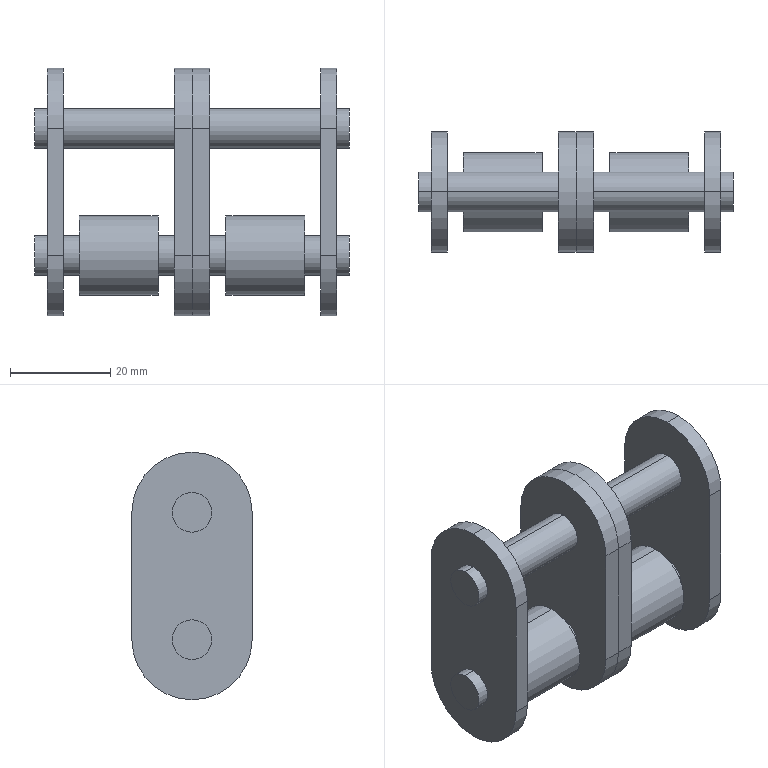Part | SolidWorks | features ICE 5, CombineBodies 2, Extrusion 1, MirrorSolid 1 | 8 solids | 64 faces | box 62.7 x 24 x 49.4 mm | volume 23910 mm3 | cylinder 40 | plane 24 | commonest cylinder face diameters 7.92 x24 24 x12 15.88 x4